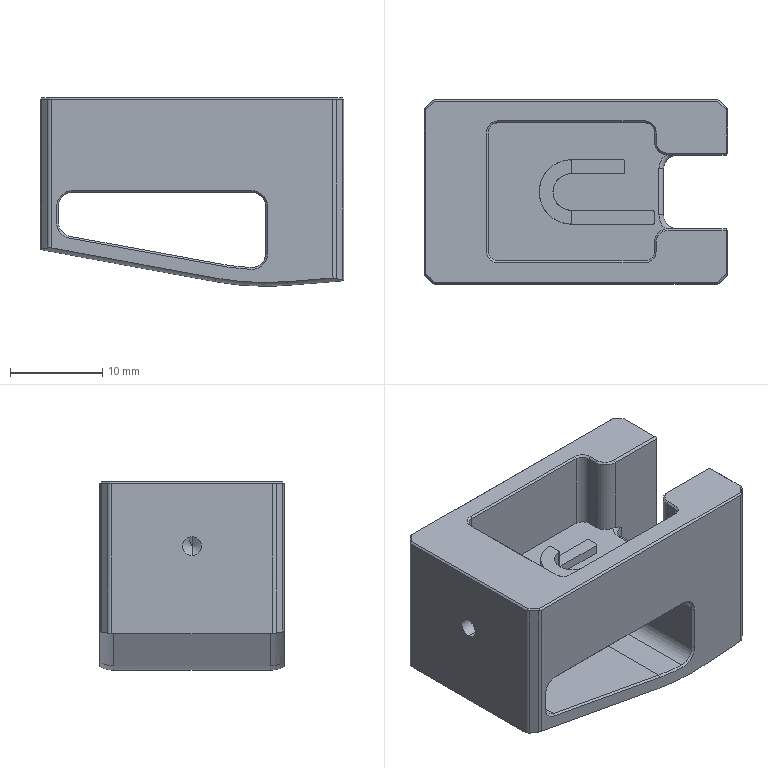NC program | NX | posted with a generic post | part box 33 x 20 x 20.478 mm
Lines 1 to 1297 of 7616:
N10 G17 G21 G94 G90
(CAVITY_MILL_1 , TOOL : D80)
N12 T19 M6
N14 G54
N16 G17 G0 G90 X95.922 Y-16.565 B0. C0. S6500 M3
N18 G43 Z30. H19
N20 Z7.
N22 G94 G1 Z4. F1500.
N24 X55.646
N26 X-55.646
N28 G2 X-56.192 Y-10.061 R39.693
N30 G1 X-56.196 Y-7.594
N32 Y7.594
N34 X-56.192 Y10.061
N36 G2 X-55.646 Y16.565 R39.693
N38 G1 X55.646
N40 X95.922
N42 Z7.
N44 G0 Z30.
N46 Y-16.565
N48 Z6.
N50 G1 Z3.
N52 X55.646
N54 X-55.646
N56 G2 X-56.192 Y-10.061 R39.693
N58 G1 X-56.196 Y-7.594
N60 Y7.594
N62 X-56.192 Y10.061
N64 G2 X-55.646 Y16.565 R39.693
N66 G1 X55.646
N68 X95.922
N70 Z6.
N72 G0 Z30.
N74 Y-16.565
N76 Z5.
N78 G1 Z2.
N80 X55.646
N82 X-55.646
N84 G2 X-56.193 Y-10.061 R39.693
N86 G1 X-56.196 Y-7.594
N88 Y7.594
N90 X-56.193 Y10.061
N92 G2 X-55.646 Y16.565 R39.693
N94 G1 X55.646
N96 X95.922
N98 Z5.
N100 G0 Z30.
N102 Y-16.565
N104 Z4.
N106 G1 Z1.
N108 X55.646
N110 X-55.646
N112 G2 X-56.193 Y-10.062 R39.693
N114 G1 X-56.196 Y-7.594
N116 Y7.594
N118 X-56.193 Y10.062
N120 G2 X-55.646 Y16.565 R39.693
N122 G1 X55.646
N124 X95.922
N126 Z4.
N128 G0 Z30.
N130 Y-16.565
N132 Z3.
N134 G1 Z0.
N136 X55.647
N138 X-55.647
N140 G2 X-56.193 Y-10.062 R39.693
N142 G1 X-56.197 Y-7.594
N144 Y7.594
N146 X-56.193 Y10.062
N148 G2 X-55.647 Y16.565 R39.693
N150 G1 X55.647
N152 X95.922
N154 Z3.
N156 G0 Z30.
N158 M5
(FIXED_CONTOUR , TOOL : D6)
N160 T12 M6
N162 G54
N164 G17 G0 G90 X-2.101 Y-13.027 B0. C0. S9500 M3
N166 G43 Z30. H12
N168 Z3.6
N170 G94 G1 Z2.384 F1000.
N172 X-2.171 Z1.918
N174 X-2.312 Z1.469
N176 X-2.522 Z1.048
N178 X-2.795 Z0.664
N180 X-3.125 Y-13.026 Z0.328
N182 X-3.503 Z0.048
N184 X-3.92 Z-0.17
N186 X-4.367 Y-13.025 Z-0.319
N188 X-4.831 Z-0.397
N190 X-5.302 Z-0.401
N192 X-5.692 Z-0.374 F2500.
N194 X-6.654 Y-13.024 Z-0.326
N196 X-7.492 Y-13.023 Z-0.305
N198 X-8.392 Z-0.304
N200 X-9.292 Y-13.022 Z-0.328
N202 X-9.487 Z-0.334
N204 X-11.092 Y-13.021 Z-0.439
N206 X-12.892 Y-13.019 Z-0.583
N208 X-14.692 Y-13.018 Z-0.728
N210 X-15.814 Y-13.017 Z-0.818
N212 X-15.995 Y-12.937 Z-0.787
N214 X-16.111 Y-12.868 Z-0.76
N216 X-16.222 Y-12.789 Z-0.733
N218 X-16.446 Y-12.623 Z-0.677
N220 X-16.548 Y-12.552 Z-0.654
N222 X-16.491 Z-0.65
N224 X-14.691 Y-12.553 Z-0.506
N226 X-12.891 Y-12.554 Z-0.362
N228 X-11.091 Y-12.556 Z-0.218
N230 X-10.191 Z-0.158
N232 X-9.291 Y-12.557 Z-0.115
N234 X-8.391 Z-0.091
N236 X-7.491 Y-12.558 Z-0.092
N238 X-6.591 Y-12.559 Z-0.116
N240 X-5.691 Z-0.158
N242 X-4.791 Y-12.56 Z-0.22
N244 X-3.891 Y-12.561 Z-0.309
N246 X-2.991 Z-0.421
N248 X-2.091 Y-12.562 Z-0.558
N250 X-0.291 Y-12.563 Z-0.878
N252 X1.509 Y-12.564 Z-1.21
N254 X3.309 Y-12.566 Z-1.541
N256 X5.109 Y-12.567 Z-1.872
N258 X6.909 Y-12.568 Z-2.203
N260 X8.709 Y-12.569 Z-2.533
N262 X10.509 Y-12.571 Z-2.864
N264 X12.309 Y-12.572 Z-3.195
N266 X14.109 Y-12.573 Z-3.525
N268 X15.909 Y-12.575 Z-3.856
N270 X16.876 Z-4.034
N272 X17.19 Y-12.346 Z-3.997
N274 X17.471 Y-12.138 Z-3.968
N276 X17.541 Y-12.083 Z-3.962
N278 X15.909 Y-12.082 Z-3.662
N280 X14.109 Y-12.081 Z-3.331
N282 X12.309 Y-12.08 Z-3.001
N284 X10.509 Y-12.078 Z-2.67
N286 X8.709 Y-12.077 Z-2.339
N288 X6.909 Y-12.076 Z-2.008
N290 X5.109 Y-12.074 Z-1.678
N292 X3.309 Y-12.073 Z-1.347
N294 X1.509 Y-12.072 Z-1.016
N296 X-0.291 Y-12.071 Z-0.685
N298 X-2.091 Y-12.069 Z-0.372
N300 X-2.991 Z-0.249
N302 X-3.891 Y-12.068 Z-0.149
N304 X-4.791 Z-0.07
N306 X-5.691 Y-12.067 Z-0.01
N308 X-7.491 Y-12.066 Z0.042
N310 X-8.391 Y-12.065 Z0.044
N312 X-9.291 Y-12.064 Z0.024
N314 X-10.191 Z-0.011
N316 X-11.091 Y-12.063 Z-0.068
N318 X-12.891 Y-12.062 Z-0.211
N320 X-14.691 Y-12.061 Z-0.355
N322 X-16.491 Y-12.059 Z-0.499
N324 X-17.269 Z-0.561
N326 X-17.674 Y-11.779 Z-0.535
N328 X-17.84 Y-11.652 Z-0.527
N330 X-17.942 Y-11.566 Z-0.522
N332 X-16.491 Y-11.567 Z-0.406
N334 X-14.691 Y-11.568 Z-0.261
N336 X-12.891 Y-11.569 Z-0.117
N338 X-11.091 Y-11.571 Z0.017
N340 X-9.291 Y-11.572 Z0.089
N342 X-7.491 Y-11.573 Z0.097
N344 X-6.591 Y-11.574 Z0.089
N346 X-5.691 Z0.06
N348 X-4.791 Y-11.575 Z0.018
N350 X-3.891 Y-11.576 Z-0.047
N352 X-2.991 Z-0.137
N354 X-2.091 Y-11.577 Z-0.251
N356 X-0.291 Y-11.578 Z-0.548
N358 X1.509 Y-11.579 Z-0.879
N360 X3.309 Y-11.581 Z-1.21
N362 X5.109 Y-11.582 Z-1.541
N364 X6.909 Y-11.583 Z-1.871
N366 X8.709 Y-11.585 Z-2.202
N368 X10.509 Y-11.586 Z-2.532
N370 X12.309 Y-11.587 Z-2.863
N372 X14.109 Y-11.588 Z-3.193
N374 X15.909 Y-11.59 Z-3.524
N376 X17.709 Y-11.591 Z-3.854
N378 X18.151 Z-3.936
N380 X18.373 Y-11.381 Z-3.929
N382 X18.575 Y-11.167 Z-3.924
N384 X18.631 Y-11.099 Z-3.922
N386 X17.71 Y-11.098 Z-3.753
N388 X15.91 Y-11.097 Z-3.423
N390 X14.11 Y-11.096 Z-3.092
N392 X12.31 Y-11.095 Z-2.762
N394 X10.51 Y-11.093 Z-2.431
N396 X8.71 Y-11.092 Z-2.101
N398 X6.91 Y-11.091 Z-1.77
N400 X5.11 Y-11.09 Z-1.44
N402 X3.31 Y-11.088 Z-1.109
N404 X1.51 Y-11.087 Z-0.779
N406 X-0.29 Y-11.086 Z-0.448
N408 X-1.19 Y-11.085 Z-0.297
N410 X-2.09 Y-11.084 Z-0.169
N412 X-2.99 Z-0.069
N414 X-3.89 Y-11.083 Z0.008
N416 X-4.79 Z0.062
N418 X-5.69 Y-11.082 Z0.091
N420 X-7.49 Y-11.081 Z0.099
N422 X-9.29 Y-11.079
N424 X-10.19 Z0.091
N426 X-11.09 Y-11.078 Z0.063
N428 X-12.89 Y-11.077 Z-0.06
N430 X-14.69 Y-11.076 Z-0.204
N432 X-16.49 Y-11.074 Z-0.348
N434 X-18.29 Y-11.073 Z-0.493
N436 X-18.439 Z-0.504
N438 X-18.508 Y-10.987 Z-0.502
N440 X-18.643 Y-10.801 Z-0.499
N442 X-18.724 Y-10.681 Z-0.496
N444 X-18.796 Y-10.58 Z-0.495
N446 X-18.29 Y-10.581 Z-0.454
N448 X-16.49 Y-10.582 Z-0.309
N450 X-14.69 Y-10.583 Z-0.165
N452 X-12.89 Y-10.584 Z-0.02
N454 X-11.99 Y-10.585 Z0.041
N456 X-11.09 Y-10.586 Z0.083
N458 X-10.19 Z0.098
N460 X-9.29 Y-10.587 Z0.099
N462 X-7.49 Y-10.588
N464 X-5.69 Y-10.59
N466 X-4.79 Z0.083
N468 X-3.89 Y-10.591 Z0.042
N470 X-2.99 Z-0.022
N472 X-2.09 Y-10.592 Z-0.113
N474 X-1.19 Y-10.593 Z-0.233
N476 X-0.29 Z-0.377
N478 X1.51 Y-10.595 Z-0.704
N480 X3.31 Y-10.596 Z-1.034
N482 X5.11 Y-10.597 Z-1.365
N484 X6.91 Y-10.598 Z-1.695
N486 X8.71 Y-10.6 Z-2.026
N488 X10.51 Y-10.601 Z-2.356
N490 X12.31 Y-10.602 Z-2.687
N492 X14.11 Y-10.603 Z-3.018
N494 X15.91 Y-10.605 Z-3.348
N496 X17.71 Y-10.606 Z-3.679
N498 X18.956 Y-10.607 Z-3.907
N500 X19.127 Y-10.287 Z-3.902
N502 X19.163 Y-10.196 Z-3.899
N504 X19.189 Y-10.115 Z-3.897
N506 X17.71 Y-10.113 Z-3.625
N508 X15.91 Y-10.112 Z-3.295
N510 X14.11 Y-10.111 Z-2.965
N512 X12.31 Y-10.11 Z-2.635
N514 X10.51 Y-10.108 Z-2.304
N516 X8.71 Y-10.107 Z-1.974
N518 X6.91 Y-10.106 Z-1.644
N520 X5.11 Y-10.105 Z-1.313
N522 X3.31 Y-10.103 Z-0.982
N524 X1.51 Y-10.102 Z-0.651
N526 X-0.29 Y-10.101 Z-0.328
N528 X-1.19 Y-10.1 Z-0.19
N530 X-2.09 Z-0.08
N532 X-2.99 Y-10.099 Z0.003
N534 X-3.89 Y-10.098 Z0.062
N536 X-4.79 Z0.092
N538 X-5.69 Y-10.097 Z0.099
N540 X-7.49 Y-10.096
N542 X-9.29 Y-10.095
N544 X-10.19 Y-10.094
N546 X-11.09 Y-10.093 Z0.093
N548 X-11.99 Z0.062
N550 X-12.89 Y-10.092 Z0.004
N552 X-14.69 Y-10.091 Z-0.138
N554 X-16.49 Y-10.089 Z-0.283
N556 X-18.29 Y-10.088 Z-0.427
N558 X-19.101 Z-0.492
N560 X-19.194 Y-9.729 Z-0.487
N562 X-19.234 Y-9.595 Z-0.486
N564 X-18.289 Y-9.596 Z-0.41
N566 X-16.489 Y-9.597 Z-0.265
N568 X-14.689 Y-9.598 Z-0.121
N570 X-12.889 Y-9.6 Z0.019
N572 X-11.989 Z0.073
N574 X-11.089 Y-9.601 Z0.097
N576 X-9.289 Y-9.602 Z0.099
N578 X-7.489 Y-9.603
N580 X-5.689 Y-9.605
N582 X-4.789 Z0.097
N584 X-3.889 Y-9.606 Z0.072
N586 X-2.989 Z0.019
N588 X-2.089 Y-9.607 Z-0.057
N590 X-1.189 Y-9.608 Z-0.162
N592 X-0.289 Z-0.294
N594 X1.511 Y-9.61 Z-0.614
N596 X3.311 Y-9.611 Z-0.944
N598 X5.111 Y-9.612 Z-1.275
N600 X6.911 Y-9.613 Z-1.605
N602 X8.711 Y-9.615 Z-1.936
N604 X10.511 Y-9.616 Z-2.266
N606 X12.311 Y-9.617 Z-2.597
N608 X14.111 Y-9.618 Z-2.927
N610 X15.911 Y-9.62 Z-3.258
N612 X17.711 Y-9.621 Z-3.588
N614 X19.336 Y-9.622 Z-3.886
N616 X19.428 Y-9.225 Z-3.884
N618 X19.439 Y-9.13 Z-3.883
N620 X17.711 Y-9.129 Z-3.566
N622 X15.911 Y-9.127 Z-3.235
N624 X14.111 Y-9.126 Z-2.905
N626 X12.311 Y-9.125 Z-2.575
N628 X10.511 Y-9.124 Z-2.244
N630 X8.711 Y-9.122 Z-1.914
N632 X6.911 Y-9.121 Z-1.584
N634 X5.111 Y-9.12 Z-1.254
N636 X3.311 Y-9.118 Z-0.923
N638 X1.511 Y-9.117 Z-0.593
N640 X-0.289 Y-9.116 Z-0.274
N642 X-1.189 Y-9.115 Z-0.144
N644 X-2.089 Z-0.042
N646 X-2.989 Y-9.114 Z0.029
N648 X-3.889 Y-9.113 Z0.078
N650 X-4.789 Z0.099
N652 X-5.689 Y-9.112
N654 X-7.489 Y-9.111
N656 X-9.289 Y-9.11
N658 X-11.089 Y-9.108 Z0.098
N660 X-11.989 Z0.079
N662 X-12.889 Y-9.107 Z0.029
N664 X-14.689 Y-9.106 Z-0.109
N666 X-16.489 Y-9.105 Z-0.254
N668 X-18.289 Y-9.103 Z-0.399
N670 X-19.371 Z-0.486
N672 X-19.482 Y-8.61 Z-0.49
N674 X-18.289 Y-8.611 Z-0.394
N676 X-16.489 Y-8.612 Z-0.249
N678 X-14.689 Y-8.613 Z-0.105
N680 X-12.889 Y-8.615 Z0.033
N682 X-11.989 Z0.081
N684 X-11.089 Y-8.616 Z0.098
N686 X-9.289 Y-8.617 Z0.099
N688 X-7.489 Y-8.618
N690 X-5.689 Y-8.62
N692 X-4.789
N694 X-3.889 Y-8.621 Z0.08
N696 X-2.989 Y-8.622 Z0.033
N698 X-2.089 Z-0.036
N700 X-1.189 Y-8.623 Z-0.137
N702 X-0.289 Z-0.264
N704 X1.511 Y-8.625 Z-0.582
N706 X3.311 Y-8.626 Z-0.912
N708 X5.111 Y-8.627 Z-1.242
N710 X6.911 Y-8.629 Z-1.573
N712 X8.711 Y-8.63 Z-1.903
N714 X10.511 Y-8.631 Z-2.234
N716 X12.311 Y-8.632 Z-2.564
N718 X14.111 Y-8.634 Z-2.895
N720 X15.911 Y-8.635 Z-3.225
N722 X17.711 Y-8.636 Z-3.555
N724 X19.491 Y-8.637 Z-3.882
N726 X19.512 Y-8.254 Z-3.885
N728 Y-8.145
N730 X0.499 Y-8.132 Z-0.395
N732 X-0.288 Y-8.131 Z-0.264
N734 X-1.188 Y-8.13 Z-0.136
N736 X-2.088 Z-0.035
N738 X-2.988 Y-8.129 Z0.033
N740 X-3.888 Y-8.128 Z0.08
N742 X-4.788 Z0.099
N744 X-5.688 Y-8.127
N746 X-7.488 Y-8.126
N748 X-9.288 Y-8.125
N750 X-11.088 Y-8.123 Z0.098
N752 X-11.988 Z0.081
N754 X-12.888 Y-8.122 Z0.033
N756 X-13.359 Z0.003
N758 X-19.508 Y-8.117 Z-0.492
N760 Y-7.625
N762 X-13.359 Y-7.629 Z0.003
N764 X-12.888 Y-7.63 Z0.033
N766 X-11.988 Z0.081
N768 X-11.088 Y-7.631 Z0.098
N770 X-9.288 Y-7.632 Z0.099
N772 X-7.488 Y-7.633
N774 X-5.688 Y-7.635
N776 X-4.788
N778 X-3.888 Y-7.636 Z0.08
N780 X-2.988 Y-7.637 Z0.033
N782 X-2.088 Z-0.036
N784 X-1.188 Y-7.638 Z-0.136
N786 X-0.288 Y-7.639 Z-0.264
N788 X0.5 Z-0.395
N790 X19.512 Y-7.652 Z-3.885
N792 Y-7.16
N794 X0.5 Y-7.147 Z-0.396
N796 X-0.288 Y-7.146 Z-0.264
N798 X-1.188 Y-7.145 Z-0.136
N800 X-2.088 Z-0.036
N802 X-2.988 Y-7.144 Z0.033
N804 X-3.888 Z0.08
N806 X-4.788 Y-7.143 Z0.099
N808 X-5.688 Y-7.142
N810 X-7.488 Y-7.141
N812 X-9.288 Y-7.14
N814 X-11.088 Y-7.138 Z0.098
N816 X-11.988 Z0.081
N818 X-12.888 Y-7.137 Z0.033
N820 X-13.359 Z0.003
N822 X-19.507 Y-7.133 Z-0.492
N824 Y-6.64
N826 X-13.358 Y-6.644 Z0.003
N828 X-12.887 Y-6.645 Z0.033
N830 X-11.987 Z0.081
N832 X-11.087 Y-6.646 Z0.098
N834 X-9.287 Y-6.647 Z0.099
N836 X-7.487 Y-6.649
N838 X-5.687 Y-6.65
N840 X-4.787
N842 X-3.887 Y-6.651 Z0.08
N844 X-2.987 Y-6.652 Z0.033
N846 X-2.087 Z-0.036
N848 X-1.187 Y-6.653 Z-0.136
N850 X-0.287 Y-6.654 Z-0.264
N852 X0.5 Z-0.396
N854 X19.512 Y-6.668 Z-3.885
N856 Y-6.175
N858 X0.501 Y-6.162 Z-0.396
N860 X-0.287 Y-6.161 Z-0.264
N862 X-1.187 Z-0.137
N864 X-2.087 Y-6.16 Z-0.036
N866 X-2.987 Y-6.159 Z0.033
N868 X-3.887 Z0.08
N870 X-4.787 Y-6.158 Z0.099
N872 X-5.687 Y-6.157
N874 X-7.487 Y-6.156
N876 X-9.287 Y-6.155
N878 X-11.087 Y-6.154 Z0.098
N880 X-11.987 Y-6.153 Z0.081
N882 X-12.887 Y-6.152 Z0.033
N884 X-13.358 Z0.003
N886 X-19.507 Y-6.148 Z-0.492
N888 Y-5.655
N890 X-13.358 Y-5.66 Z0.003
N892 X-12.887 Z0.032
N894 X-11.987 Z0.081
N896 X-11.087 Y-5.661 Z0.098
N898 X-9.287 Y-5.662 Z0.099
N900 X-7.487 Y-5.664
N902 X-5.687 Y-5.665
N904 X-4.787 Y-5.666
N906 X-3.887 Z0.08
N908 X-2.987 Y-5.667 Z0.033
N910 X-2.087 Z-0.036
N912 X-1.187 Y-5.668 Z-0.137
N914 X-0.287 Y-5.669 Z-0.264
N916 X0.501 Z-0.396
N918 X19.512 Y-5.683 Z-3.885
N920 Y-5.19
N922 X0.501 Y-5.177 Z-0.396
N924 X-0.286 Y-5.176 Z-0.264
N926 X-1.186 Z-0.137
N928 X-2.086 Y-5.175 Z-0.036
N930 X-2.986 Y-5.174 Z0.033
N932 X-3.886 Z0.08
N934 X-4.786 Y-5.173 Z0.099
N936 X-5.686 Y-5.172
N938 X-7.486 Y-5.171
N940 X-9.286 Y-5.17
N942 X-11.086 Y-5.169 Z0.098
N944 X-11.986 Y-5.168 Z0.081
N946 X-12.886 Y-5.167 Z0.034
N948 X-13.357 Z0.003
N950 X-19.507 Y-5.163 Z-0.492
N952 X-19.506 Y-4.855
N954 X-19.502 Y-4.67
N956 X-13.357 Y-4.675 Z0.003
N958 X-12.886 Z0.036
N960 X-11.986 Y-4.676 Z0.082
N962 X-11.086 Z0.098
N964 X-9.286 Y-4.677 Z0.099
N966 X-7.486 Y-4.679
N968 X-5.686 Y-4.68
N970 X-4.786 Y-4.681
N972 X-3.886 Z0.08
N974 X-2.986 Y-4.682 Z0.033
N976 X-2.086 Y-4.683 Z-0.036
N978 X-1.186 Z-0.137
N980 X-0.286 Y-4.684 Z-0.264
N982 X0.502 Z-0.396
N984 X19.512 Y-4.698 Z-3.885
N986 Y-4.205
N988 X0.502 Y-4.192 Z-0.396
N990 X-0.286 Y-4.191 Z-0.264
N992 X-1.186 Z-0.137
N994 X-2.086 Y-4.19 Z-0.036
N996 X-2.986 Y-4.189 Z0.033
N998 X-3.886 Z0.08
N1000 X-4.786 Y-4.188 Z0.099
N1002 X-5.686
N1004 X-7.486 Y-4.186
N1006 X-9.286 Y-4.185
N1008 X-11.086 Y-4.184 Z0.098
N1010 X-11.986 Y-4.183 Z0.082
N1012 X-12.886 Y-4.182 Z0.037
N1014 X-13.448 Z-0.006
N1016 X-14.686 Y-4.181 Z-0.106
N1018 X-16.486 Y-4.18 Z-0.251
N1020 X-18.286 Y-4.179 Z-0.395
N1022 X-19.478 Y-4.178 Z-0.491
N1024 X-19.473 Y-4.126 Z-0.492
N1026 X-19.43 Y-3.884
N1028 X-19.376 Y-3.685 Z-0.491
N1030 X-18.285 Y-3.686 Z-0.404
N1032 X-16.485 Y-3.687 Z-0.259
N1034 X-14.685 Y-3.689 Z-0.114
N1036 X-13.785 Z-0.041
N1038 X-12.885 Y-3.69 Z0.034
N1040 X-11.985 Y-3.691 Z0.082
N1042 X-11.085 Z0.098
N1044 X-9.285 Y-3.693 Z0.099
N1046 X-7.485 Y-3.694
N1048 X-5.685 Y-3.695
N1050 X-4.785 Y-3.696
N1052 X-3.885 Z0.08
N1054 X-2.985 Y-3.697 Z0.033
N1056 X-2.085 Y-3.698 Z-0.036
N1058 X-1.185 Z-0.137
N1060 X-0.285 Y-3.699 Z-0.265
N1062 X0.495 Z-0.395
N1064 X19.512 Y-3.713 Z-3.885
N1066 Y-3.22
N1068 X0.496 Y-3.207 Z-0.395
N1070 X-0.285 Y-3.206 Z-0.265
N1072 X-1.185 Z-0.137
N1074 X-2.085 Y-3.205 Z-0.036
N1076 X-2.985 Y-3.204 Z0.033
N1078 X-3.885 Z0.08
N1080 X-4.785 Y-3.203 Z0.099
N1082 X-5.685
N1084 X-7.485 Y-3.201
N1086 X-9.285 Y-3.2
N1088 X-11.085 Y-3.199 Z0.098
N1090 X-11.985 Y-3.198 Z0.082
N1092 X-12.885 Z0.023
N1094 X-12.99 Y-3.197 Z0.013
N1096 X-13.095 Z0.003
N1098 X-13.757 Z-0.055
N1100 X-14.685 Y-3.196 Z-0.13
N1102 X-16.485 Y-3.195 Z-0.274
N1104 X-18.285 Y-3.194 Z-0.419
N1106 X-19.178 Y-3.193 Z-0.491
N1108 X-19.127 Y-3.084 Z-0.492
N1110 X-19.023 Y-2.913 Z-0.491
N1112 X-18.867 Y-2.701
N1114 X-18.285 Z-0.444
N1116 X-16.485 Y-2.703 Z-0.299
N1118 X-14.685 Y-2.704 Z-0.154
N1120 X-13.335 Y-2.705 Z-0.046
N1122 X-12.885 Z-0.004
N1124 X-12.819 Z0.003
N1126 X-12.627 Z0.024
N1128 X-12.435 Z0.044
N1130 X-11.985 Y-2.706 Z0.082
N1132 X-11.085 Z0.098
N1134 X-9.285 Y-2.708 Z0.099
N1136 X-7.485 Y-2.709
N1138 X-5.685 Y-2.71
N1140 X-4.785 Y-2.711
N1142 X-3.885 Z0.08
N1144 X-2.985 Y-2.712 Z0.032
N1146 X-2.085 Y-2.713 Z-0.036
N1148 X-1.185 Z-0.137
N1150 X-0.285 Y-2.714 Z-0.265
N1152 X0.496 Z-0.395
N1154 X19.512 Y-2.728 Z-3.885
N1156 Y-2.235
N1158 X0.496 Y-2.222 Z-0.395
N1160 X-0.284 Y-2.221 Z-0.265
N1162 X-1.184 Z-0.137
N1164 X-2.084 Y-2.22 Z-0.036
N1166 X-2.984 Z0.032
N1168 X-3.884 Y-2.219 Z0.08
N1170 X-4.784 Y-2.218 Z0.099
N1172 X-5.684
N1174 X-7.484 Y-2.216
N1176 X-9.284 Y-2.215
N1178 X-11.084 Y-2.214 Z0.098
N1180 X-11.744 Y-2.213 Z0.088
N1182 X-11.992 Z0.081
N1184 X-12.045 Z0.056
N1186 X-12.074 Z0.051
N1188 X-12.239 Z0.025
N1190 X-12.404 Z0.002
N1192 X-12.884 Z-0.048
N1194 X-14.684 Y-2.211 Z-0.193
N1196 X-16.484 Y-2.21 Z-0.338
N1198 X-18.284 Y-2.209 Z-0.483
N1200 X-18.375 Z-0.49
N1202 X-18.159 Y-2.031 Z-0.492
N1204 X-18.024 Y-1.942
N1206 X-17.674 Y-1.77
N1208 X-17.53 Y-1.717 Z-0.49
N1210 X-16.484 Y-1.718 Z-0.406
N1212 X-14.684 Y-1.719 Z-0.261
N1214 X-12.884 Y-1.72 Z-0.116
N1216 X-12.158 Y-1.721 Z-0.058
N1218 X-12.091 Z0.01
N1220 X-12.049 Z0.052
N1222 X-12.041 Z0.059
N1224 X-12.024 Z0.07
N1226 X-11.99 Z0.081
N1228 X-11.621 Z0.091
N1230 X-11.084 Z0.098
N1232 X-9.284 Y-1.723 Z0.099
N1234 X-7.484 Y-1.724
N1236 X-5.684 Y-1.725
N1238 X-4.784 Y-1.726
N1240 X-3.884 Z0.08
N1242 X-2.984 Y-1.727 Z0.032
N1244 X-2.084 Y-1.728 Z-0.036
N1246 X-1.184 Z-0.137
N1248 X-0.284 Y-1.729 Z-0.265
N1250 X0.497 Y-1.73 Z-0.395
N1252 X19.512 Y-1.743 Z-3.885
N1254 Y-1.25
N1256 X0.497 Y-1.237 Z-0.395
N1258 X-0.283 Z-0.265
N1260 X-1.183 Y-1.236 Z-0.137
N1262 X-2.083 Y-1.235 Z-0.036
N1264 X-2.983 Z0.032
N1266 X-3.883 Y-1.234 Z0.08
N1268 X-4.783 Y-1.233 Z0.099
N1270 X-5.683
N1272 X-7.483 Y-1.231
N1274 X-9.283 Y-1.23
N1276 X-11.083 Y-1.229 Z0.098
N1278 X-11.805 Y-1.228 Z0.086
N1280 X-11.986 Z0.082
N1282 X-12.031 Z0.067
N1284 X-12.053 Z0.048
N1286 X-12.527 Z-0.426
N1288 X-16.733 Y-1.225 Z-0.767
N1290 X-16.682 Y-1.005 Z-0.977
N1292 X-16.494 Y-0.951 Z-1.014
N1294 X-12.6 Y-0.941 Z-0.711
N1296 X-12.597 Y-1.149 Z-0.508
N1298 X-12.571 Y-1.189 Z-0.468
N1300 Y-1.186 Z-0.47
N1302 Y-0.735
N1304 X-12.052 Y-0.736 Z0.049
N1306 X-12.046 Z0.054
N1308 X-12. Z0.079
N1310 X-11.977 Z0.082
N1312 X-11.955 Z0.083
N1314 X-11.083 Y-0.737 Z0.098
N1316 X-9.283 Y-0.738 Z0.099
N1318 X-7.483 Y-0.739
N1320 X-5.683 Y-0.74
N1322 X-4.783 Y-0.741
N1324 X-3.883 Y-0.742 Z0.08
N1326 X-2.983 Z0.032
N1328 X-2.083 Y-0.743 Z-0.036
N1330 X-1.183 Z-0.137
N1332 X-0.283 Y-0.744 Z-0.265
N1334 X0.497 Y-0.745 Z-0.395
N1336 X19.512 Y-0.758 Z-3.885
N1338 Y-0.266
N1340 X0.498 Y-0.252 Z-0.395
N1342 X-0.283 Z-0.265
N1344 X-1.183 Y-0.251 Z-0.137
N1346 X-2.083 Y-0.25 Z-0.036
N1348 X-2.983 Z0.032
N1350 X-3.883 Y-0.249 Z0.08
N1352 X-4.783 Y-0.248 Z0.099
N1354 X-5.683
N1356 X-7.483 Y-0.247
N1358 X-9.283 Y-0.245
N1360 X-11.083 Y-0.244 Z0.098
N1362 X-11.977 Y-0.243 Z0.082
N1364 X-12. Z0.079
N1366 X-12.046 Z0.055
N1368 X-12.052 Z0.049
N1370 X-12.566 Z-0.465
N1372 X-12.571 Z-0.47
N1374 Y0.249
N1376 X-12.052 Z0.049
N1378 X-12.046 Z0.055
N1380 X-12. Z0.079
N1382 X-11.977 Z0.082
N1384 X-11.954 Z0.083
N1386 X-11.082 Y0.248 Z0.098
N1388 X-9.282 Y0.247 Z0.099
N1390 X-7.482 Y0.246
N1392 X-5.682 Y0.245
N1394 X-4.782 Y0.244
N1396 X-3.882 Y0.243 Z0.08
N1398 X-2.982 Z0.032
N1400 X-2.082 Y0.242 Z-0.036
N1402 X-1.182 Y0.241 Z-0.137
N1404 X-0.282 Z-0.265
N1406 X0.498 Y0.24 Z-0.395
N1408 X19.512 Y0.227 Z-3.885
N1410 Y0.719
N1412 X0.498 Y0.733 Z-0.395
N1414 X-0.282 Z-0.265
N1416 X-1.182 Y0.734 Z-0.137
N1418 X-2.082 Y0.735 Z-0.036
N1420 X-2.982 Z0.032
N1422 X-3.882 Y0.736 Z0.08
N1424 X-4.782 Z0.099
N1426 X-5.682 Y0.737
N1428 X-7.482 Y0.738
N1430 X-9.282 Y0.74
N1432 X-11.082 Y0.741 Z0.098
N1434 X-11.977 Y0.742 Z0.082
N1436 X-12. Z0.079
N1438 X-12.046 Z0.055
N1440 X-12.052 Z0.049
N1442 X-12.566 Z-0.465
N1444 X-12.571 Z-0.47
N1446 Y1.147
N1448 X-12.574 Y1.183 Z-0.473
N1450 X-12.577 Y1.196 Z-0.462
N1452 X-12.597 Y1.139 Z-0.518
N1454 X-12.6 Y0.941 Z-0.711
N1456 X-16.403 Y0.948 Z-1.009
N1458 X-16.677 Y0.988 Z-0.994
N1460 X-16.735 Y1.237 Z-0.755
N1462 X-12.52 Y1.234 Z-0.419
N1464 X-12.048 Z0.053
N1466 X-12.026 Z0.07
N1468 X-12.003 Z0.079
N1470 X-11.992 Z0.081
N1472 X-11.981 Z0.082
N1474 X-11.801 Z0.086
N1476 X-11.082 Y1.233 Z0.098
N1478 X-9.282 Y1.232 Z0.099
N1480 X-7.482 Y1.231
N1482 X-5.682 Y1.23
N1484 X-4.782 Y1.229
N1486 X-3.882 Y1.228 Z0.08
N1488 X-2.982 Z0.032
N1490 X-2.082 Y1.227 Z-0.036
N1492 X-1.182 Y1.226 Z-0.137
N1494 X-0.282 Z-0.265
N1496 X0.499 Y1.225 Z-0.395
N1498 X19.512 Y1.212 Z-3.885
N1500 Y1.704
N1502 X0.499 Y1.718 Z-0.395
N1504 X-0.281 Z-0.265
N1506 X-1.181 Y1.719 Z-0.137
N1508 X-2.081 Z-0.036
N1510 X-2.981 Y1.72 Z0.032
N1512 X-3.881 Y1.721 Z0.08
N1514 X-4.781 Z0.099
N1516 X-5.681 Y1.722
N1518 X-7.481 Y1.723
N1520 X-9.281 Y1.725
N1522 X-11.081 Y1.726 Z0.098
N1524 X-11.981 Z0.082
N1526 X-12.025 Z0.07
N1528 X-12.047 Z0.054
N1530 X-12.053 Z0.048
N1532 X-12.157 Y1.727 Z-0.056
N1534 X-12.881 Z-0.114
N1536 X-14.681 Y1.728 Z-0.259
N1538 X-16.481 Y1.73 Z-0.403
N1540 X-17.572 Z-0.491
N1542 X-17.674 Y1.767 Z-0.492
N1544 X-17.851 Y1.849
N1546 X-18.025 Y1.942
N1548 X-18.159 Y2.028
N1550 X-18.41 Y2.223 Z-0.491
N1552 X-18.281 Z-0.481
N1554 X-16.481 Y2.222 Z-0.336
N1556 X-14.681 Y2.221 Z-0.192
N1558 X-12.881 Y2.22 Z-0.047
N1560 X-12.431 Y2.219 Z-0.001
N1562 X-12.392 Z0.005
N1564 X-12.206 Z0.03
N1566 X-12.094 Z0.048
N1568 X-12.044 Z0.057
N1570 X-12.037 Z0.062
N1572 X-11.981 Z0.082
N1574 X-11.081 Y2.218 Z0.098
N1576 X-9.281 Y2.217 Z0.099
N1578 X-7.481 Y2.216
N1580 X-5.681 Y2.214
N1582 X-4.781
N1584 X-3.881 Y2.213 Z0.08
N1586 X-2.981 Z0.032
N1588 X-2.081 Y2.212 Z-0.036
N1590 X-1.181 Y2.211 Z-0.137
N1592 X-0.281 Z-0.265
N1594 X0.499 Y2.21 Z-0.395
N1596 X19.512 Y2.197 Z-3.885
N1598 Y2.689
N1600 X0.5 Y2.703 Z-0.395
N1602 X-0.281 Z-0.265
N1604 X-1.181 Y2.704 Z-0.137
N1606 X-2.081 Z-0.036
N1608 X-2.981 Y2.705 Z0.032
N1610 X-3.881 Y2.706 Z0.08
N1612 X-4.781 Z0.099
N1614 X-5.681 Y2.707
N1616 X-7.481 Y2.708
N1618 X-9.281 Y2.709
N1620 X-11.081 Y2.711 Z0.098
N1622 X-12.009 Z0.081
N1624 X-12.206 Y2.712 Z0.066
N1626 X-12.81 Z0.005
N1628 X-12.881 Z-0.003
N1630 X-14.681 Y2.713 Z-0.153
N1632 X-16.481 Y2.715 Z-0.298
N1634 X-18.281 Y2.716 Z-0.443
N1636 X-18.879 Z-0.491
N1638 X-19.023 Y2.913
N1640 X-19.127 Y3.083 Z-0.492
N1642 X-19.191 Y3.209
N1644 X-18.28 Y3.208 Z-0.418
N1646 X-16.48 Y3.207 Z-0.274
N1648 X-14.68 Y3.206 Z-0.129
N1650 X-13.78 Y3.205 Z-0.056
N1652 X-13.33 Z-0.018
N1654 X-12.88 Y3.204 Z0.023
N1656 X-12.43 Z0.06
N1658 X-12.093 Z0.078
N1660 X-11.98 Z0.082
N1662 X-11.08 Y3.203 Z0.098
N1664 X-9.28 Y3.202 Z0.099
N1666 X-7.48 Y3.201
N1668 X-5.68 Y3.199
N1670 X-4.78
N1672 X-3.88 Y3.198 Z0.08
N1674 X-2.98 Y3.197 Z0.032
N1676 X-2.08 Z-0.036
N1678 X-1.18 Y3.196 Z-0.137
N1680 X-0.28 Z-0.265
N1682 X0.5 Y3.195 Z-0.396
N1684 X19.512 Y3.182 Z-3.885
N1686 Y3.674
N1688 X0.5 Y3.688 Z-0.396
N1690 X-0.28 Z-0.265
N1692 X-1.18 Y3.689 Z-0.137
N1694 X-2.08 Z-0.036
N1696 X-2.98 Y3.69 Z0.032
N1698 X-3.88 Y3.691 Z0.08
N1700 X-4.78 Z0.099
N1702 X-5.68 Y3.692
N1704 X-7.48 Y3.693
N1706 X-9.28 Y3.694
N1708 X-11.08 Y3.696 Z0.098
N1710 X-11.98 Z0.081
N1712 X-12.43 Y3.697 Z0.063
N1714 X-12.88 Z0.034
N1716 X-13.78 Y3.698 Z-0.041
N1718 X-14.68 Z-0.113
N1720 X-16.48 Y3.699 Z-0.258
N1722 X-18.28 Y3.701 Z-0.403
N1724 X-19.38 Z-0.491
N1726 X-19.43 Y3.884 Z-0.492
N1728 X-19.473 Y4.126
N1730 X-19.479 Y4.194 Z-0.491
N1732 X-18.28 Y4.193 Z-0.395
N1734 X-16.48 Y4.192 Z-0.25
N1736 X-14.68 Y4.191 Z-0.105
N1738 X-13.105 Y4.19 Z0.022
N1740 X-12.88 Y4.189 Z0.037
N1742 X-11.98 Z0.081
N1744 X-11.08 Y4.188 Z0.098
N1746 X-9.28 Y4.187 Z0.099
N1748 X-7.48 Y4.186
N1750 X-5.68 Y4.184
N1752 X-4.78
N1754 X-3.88 Y4.183 Z0.08
N1756 X-2.98 Y4.182 Z0.032
N1758 X-2.08 Z-0.036
N1760 X-1.18 Y4.181 Z-0.137
N1762 X-0.28 Z-0.265
N1764 X0.501 Y4.18 Z-0.396
N1766 X19.512 Y4.167 Z-3.885
N1768 Y4.659
N1770 X0.501 Y4.672 Z-0.396
N1772 X-0.279 Y4.673 Z-0.266
N1774 X-1.179 Y4.674 Z-0.138
N1776 X-2.079 Z-0.036
N1778 X-2.979 Y4.675 Z0.032
N1780 X-3.879 Z0.08
N1782 X-4.779 Y4.676 Z0.099
N1784 X-5.679 Y4.677
N1786 X-7.479 Y4.678
N1788 X-9.279 Y4.679
N1790 X-11.079 Y4.681 Z0.098
N1792 X-11.979 Z0.081
N1794 X-12.879 Y4.682 Z0.036
N1796 X-13.357 Z0.003
N1798 X-19.502 Y4.686 Z-0.492
N1800 X-19.506 Y4.855
N1802 X-19.507 Y5.179
N1804 X-13.357 Y5.175 Z0.003
N1806 X-12.879 Y5.174 Z0.035
N1808 X-11.979 Z0.081
N1810 X-11.079 Y5.173 Z0.098
N1812 X-9.279 Y5.172 Z0.099
N1814 X-7.479 Y5.17
N1816 X-5.679 Y5.169
N1818 X-4.779
N1820 X-3.879 Y5.168 Z0.08
N1822 X-2.979 Y5.167 Z0.032
N1824 X-2.079 Z-0.036
N1826 X-1.179 Y5.166 Z-0.138
N1828 X-0.279 Y5.165 Z-0.266
N1830 X0.501 Z-0.396
N1832 X19.512 Y5.152 Z-3.885
N1834 Y5.644
N1836 X0.502 Y5.657 Z-0.396
N1838 X-0.279 Y5.658 Z-0.266
N1840 X-1.179 Y5.659 Z-0.138
N1842 X-2.079 Z-0.037
N1844 X-2.979 Y5.66 Z0.032
N1846 X-3.879 Z0.08
N1848 X-4.779 Y5.661 Z0.099
N1850 X-5.679 Y5.662
N1852 X-7.479 Y5.663
N1854 X-9.279 Y5.664
N1856 X-11.079 Y5.665 Z0.098
N1858 X-11.979 Y5.666 Z0.081
N1860 X-12.879 Y5.667 Z0.034
N1862 X-13.357 Z0.003
N1864 X-19.507 Y5.671 Z-0.492
N1866 Y6.164
N1868 X-13.356 Y6.16 Z0.003
N1870 X-12.878 Y6.159 Z0.034
N1872 X-11.978 Z0.081
N1874 X-11.078 Y6.158 Z0.098
N1876 X-9.278 Y6.157 Z0.099
N1878 X-7.478 Y6.155
N1880 X-5.678 Y6.154
N1882 X-4.778
N1884 X-3.878 Y6.153 Z0.08
N1886 X-2.978 Y6.152 Z0.032
N1888 X-2.078 Z-0.037
N1890 X-1.178 Y6.151 Z-0.138
N1892 X-0.278 Y6.15 Z-0.266
N1894 X0.495 Z-0.395
N1896 X19.512 Y6.136 Z-3.885
N1898 Y6.629
N1900 X0.495 Y6.642 Z-0.395
N1902 X-0.278 Y6.643 Z-0.266
N1904 X-1.178 Z-0.138
N1906 X-2.078 Y6.644 Z-0.037
N1908 X-2.978 Y6.645 Z0.032
N1910 X-3.878 Z0.08
N1912 X-4.778 Y6.646 Z0.099
N1914 X-5.678 Y6.647
N1916 X-7.478 Y6.648
N1918 X-9.278 Y6.649
N1920 X-11.078 Y6.65 Z0.098
N1922 X-11.978 Y6.651 Z0.081
N1924 X-12.878 Y6.652 Z0.033
N1926 X-13.356 Z0.003
N1928 X-19.507 Y6.656 Z-0.492
N1930 Y7.149
N1932 X-13.356 Y7.144 Z0.003
N1934 X-12.878 Z0.034
N1936 X-11.978 Y7.143 Z0.081
N1938 X-11.078 Z0.098
N1940 X-9.278 Y7.142 Z0.099
N1942 X-7.478 Y7.14
N1944 X-5.678 Y7.139
N1946 X-4.778 Y7.138
N1948 X-3.878 Z0.08
N1950 X-2.978 Y7.137 Z0.032
N1952 X-2.078 Z-0.037
N1954 X-1.178 Y7.136 Z-0.138
N1956 X-0.278 Y7.135 Z-0.266
N1958 X0.496 Z-0.395
N1960 X19.512 Y7.121 Z-3.885
N1962 Y7.614
N1964 X0.496 Y7.627 Z-0.395
N1966 X-0.277 Y7.628 Z-0.266
N1968 X-1.177 Z-0.138
N1970 X-2.077 Y7.629 Z-0.037
N1972 X-2.977 Y7.63 Z0.032
N1974 X-3.877 Z0.08
N1976 X-4.777 Y7.631 Z0.099
N1978 X-5.677 Y7.632
N1980 X-7.477 Y7.633
N1982 X-9.277 Y7.634
N1984 X-11.077 Y7.635 Z0.098
N1986 X-11.977 Y7.636 Z0.081
N1988 X-12.877 Y7.637 Z0.034
N1990 X-13.355 Z0.003
N1992 X-19.508 Y7.641 Z-0.492
N1994 Y8.134
N1996 X-13.355 Y8.129 Z0.003
N1998 X-12.877 Z0.034
N2000 X-11.977 Y8.128 Z0.081
N2002 X-11.077 Z0.098
N2004 X-9.277 Y8.127 Z0.099
N2006 X-7.477 Y8.125
N2008 X-5.677 Y8.124
N2010 X-4.777 Y8.123
N2012 X-3.877 Z0.08
N2014 X-2.977 Y8.122 Z0.032
N2016 X-2.077 Y8.121 Z-0.037
N2018 X-1.177 Z-0.138
N2020 X-0.277 Y8.12 Z-0.266
N2022 X0.497 Z-0.395
N2024 X19.512 Y8.106 Z-3.885
N2026 Y8.254
N2028 X19.493 Y8.599 Z-3.882
N2030 X17.723 Y8.6 Z-3.557
N2032 X15.923 Y8.601 Z-3.227
N2034 X14.123 Y8.603 Z-2.897
N2036 X12.323 Y8.604 Z-2.566
N2038 X10.523 Y8.605 Z-2.236
N2040 X8.723 Y8.606 Z-1.905
N2042 X6.923 Y8.608 Z-1.575
N2044 X5.123 Y8.609 Z-1.245
N2046 X3.323 Y8.61 Z-0.914
N2048 X1.523 Y8.611 Z-0.584
N2050 X-0.277 Y8.613 Z-0.266
N2052 X-1.177 Z-0.138
N2054 X-2.077 Y8.614 Z-0.037
N2056 X-2.977 Y8.615 Z0.032
N2058 X-3.877 Z0.08
N2060 X-4.777 Y8.616 Z0.099
N2062 X-5.677
N2064 X-7.477 Y8.618
N2066 X-9.277 Y8.619
N2068 X-11.077 Y8.62 Z0.098
N2070 X-11.977 Y8.621 Z0.081
N2072 X-12.877 Y8.622 Z0.033
N2074 X-14.677 Y8.623 Z-0.104
N2076 X-16.477 Y8.624 Z-0.248
N2078 X-18.277 Y8.625 Z-0.393
N2080 X-19.478 Y8.626 Z-0.49
N2082 X-19.367 Y9.119 Z-0.486
N2084 X-18.276 Y9.118 Z-0.398
N2086 X-16.476 Y9.116 Z-0.253
N2088 X-14.676 Y9.115 Z-0.108
N2090 X-12.876 Y9.114 Z0.03
N2092 X-11.976 Y9.113 Z0.08
N2094 X-11.076 Z0.098
N2096 X-9.276 Y9.111 Z0.099
N2098 X-7.476 Y9.11
N2100 X-5.676 Y9.109
N2102 X-4.776 Y9.108
N2104 X-3.876 Z0.077
N2106 X-2.976 Y9.107 Z0.028
N2108 X-2.076 Y9.106 Z-0.043
N2110 X-1.176 Z-0.146
N2112 X-0.276 Y9.105 Z-0.276
N2114 X1.524 Y9.104 Z-0.595
N2116 X3.324 Y9.103 Z-0.925
N2118 X5.124 Y9.101 Z-1.255
N2120 X6.924 Y9.1 Z-1.586
N2122 X8.724 Y9.099 Z-1.916
N2124 X10.524 Y9.098 Z-2.246
N2126 X12.324 Y9.096 Z-2.576
N2128 X14.124 Y9.095 Z-2.907
N2130 X15.924 Y9.094 Z-3.237
N2132 X17.724 Y9.092 Z-3.567
N2134 X19.444 Y9.091 Z-3.883
N2136 X19.428 Y9.225 Z-3.884
N2138 X19.345 Y9.584 Z-3.886
N2140 X17.724 Y9.585 Z-3.588
N2142 X15.924 Y9.586 Z-3.258
N2144 X14.124 Y9.587 Z-2.928
N2146 X12.324 Y9.589 Z-2.597
N2148 X10.524 Y9.59 Z-2.267
N2150 X8.724 Y9.591 Z-1.937
N2152 X6.924 Y9.593 Z-1.606
N2154 X5.124 Y9.594 Z-1.276
N2156 X3.324 Y9.595 Z-0.946
N2158 X1.524 Y9.596 Z-0.615
N2160 X-0.276 Y9.598 Z-0.296
N2162 X-1.176 Z-0.164
N2164 X-2.076 Y9.599 Z-0.058
N2166 X-2.976 Z0.018
N2168 X-3.876 Y9.6 Z0.071
N2170 X-4.776 Y9.601 Z0.096
N2172 X-5.676 Z0.099
N2174 X-7.476 Y9.603
N2176 X-9.276 Y9.604
N2178 X-11.076 Y9.605 Z0.097
N2180 X-11.976 Y9.606 Z0.074
N2182 X-12.876 Z0.02
N2184 X-14.676 Y9.608 Z-0.12
N2186 X-16.476 Y9.609 Z-0.265
N2188 X-18.276 Y9.61 Z-0.409
N2190 X-19.228 Y9.611 Z-0.486
N2192 X-19.199 Y9.71
N2194 X-19.097 Y10.103 Z-0.493
N2196 X-18.276 Z-0.427
N2198 X-16.476 Y10.101 Z-0.282
N2200 X-14.676 Y10.1 Z-0.138
N2202 X-12.876 Y10.099 Z0.005
N2204 X-11.976 Y10.098 Z0.062
N2206 X-11.076 Z0.093
N2208 X-10.176 Y10.097 Z0.099
N2210 X-9.276 Y10.096
N2212 X-7.476 Y10.095
N2214 X-5.676 Y10.094
N2216 X-4.776 Y10.093 Z0.092
N2218 X-3.876 Z0.062
N2220 X-2.976 Y10.092 Z0.002
N2222 X-2.076 Y10.091 Z-0.081
N2224 X-1.176 Z-0.192
N2226 X-0.276 Y10.09 Z-0.33
N2228 X1.524 Y10.089 Z-0.653
N2230 X3.324 Y10.088 Z-0.983
N2232 X5.124 Y10.086 Z-1.314
N2234 X6.924 Y10.085 Z-1.644
N2236 X8.724 Y10.084 Z-1.975
N2238 X10.524 Y10.082 Z-2.305
N2240 X12.324 Y10.081 Z-2.635
N2242 X14.124 Y10.08 Z-2.965
N2244 X15.924 Y10.079 Z-3.295
N2246 X17.724 Y10.077 Z-3.625
N2248 X19.201 Y10.076 Z-3.895
N2250 X19.163 Y10.196 Z-3.899
N2252 X19.127 Y10.287 Z-3.902
N2254 X18.976 Y10.569 Z-3.907
N2256 X17.725 Y10.57 Z-3.677
N2258 X15.925 Y10.571 Z-3.347
N2260 X14.125 Y10.572 Z-3.016
N2262 X12.325 Y10.574 Z-2.686
N2264 X10.525 Y10.575 Z-2.356
N2266 X8.725 Y10.576 Z-2.026
N2268 X6.925 Y10.577 Z-1.695
N2270 X5.125 Y10.579 Z-1.365
N2272 X3.325 Y10.58 Z-1.035
N2274 X1.525 Y10.581 Z-0.705
N2276 X-0.275 Y10.582 Z-0.379
N2278 X-1.175 Y10.583 Z-0.234
N2280 X-2.075 Y10.584 Z-0.114
N2282 X-2.975 Z-0.023
N2284 X-3.875 Y10.585 Z0.041
N2286 X-4.775 Y10.586 Z0.082
N2288 X-5.675 Z0.099
N2290 X-7.475 Y10.588
N2292 X-9.275 Y10.589
N2294 X-10.175 Z0.098
N2296 X-11.075 Y10.59 Z0.083
N2298 X-11.975 Y10.591 Z0.042
N2300 X-12.875 Z-0.019
N2302 X-14.675 Y10.593 Z-0.164
N2304 X-16.475 Y10.594 Z-0.309
N2306 X-18.275 Y10.595 Z-0.454
N2308 X-18.793 Y10.596 Z-0.496
N2310 X-18.508 Y10.987 Z-0.502
N2312 X-18.427 Y11.088 Z-0.505
N2314 X-18.275 Z-0.493
N2316 X-16.475 Y11.086 Z-0.348
N2318 X-14.675 Y11.085 Z-0.204
N2320 X-12.875 Y11.084 Z-0.059
N2322 X-11.075 Y11.083 Z0.064
N2324 X-10.175 Y11.082 Z0.091
N2326 X-9.275 Y11.081 Z0.099
N2328 X-7.475 Y11.08
N2330 X-5.675 Y11.079 Z0.091
N2332 X-4.775 Y11.078 Z0.062
N2334 X-3.875 Y11.077 Z0.007
N2336 X-2.975 Z-0.07
N2338 X-2.075 Y11.076 Z-0.17
N2340 X-1.175 Z-0.298
N2342 X-0.275 Y11.075 Z-0.449
N2344 X1.525 Y11.074 Z-0.779
N2346 X3.325 Y11.072 Z-1.109
N2348 X5.125 Y11.071 Z-1.439
N2350 X6.925 Y11.07 Z-1.77
N2352 X8.725 Y11.069 Z-2.1
N2354 X10.525 Y11.067 Z-2.43
N2356 X12.325 Y11.066 Z-2.76
N2358 X14.125 Y11.065 Z-3.09
N2360 X15.925 Y11.064 Z-3.42
N2362 X17.725 Y11.062 Z-3.75
N2364 X18.659 Z-3.921
N2366 X18.643 Y11.085 Z-3.922
N2368 X18.575 Y11.167 Z-3.924
N2370 X18.373 Y11.381 Z-3.929
N2372 X18.19 Y11.554 Z-3.934
N2374 X17.726 Y11.555 Z-3.849
N2376 X15.926 Y11.556 Z-3.519
N2378 X14.126 Y11.557 Z-3.189
N2380 X12.326 Y11.559 Z-2.859
N2382 X10.526 Y11.56 Z-2.529
N2384 X8.726 Y11.561 Z-2.199
N2386 X6.926 Y11.562 Z-1.869
N2388 X5.126 Y11.564 Z-1.539
N2390 X3.326 Y11.565 Z-1.209
N2392 X1.526 Y11.566 Z-0.879
N2394 X-0.274 Y11.567 Z-0.549
N2396 X-2.074 Y11.569 Z-0.252
N2398 X-2.974 Z-0.138
N2400 X-3.874 Y11.57 Z-0.048
N2402 X-4.774 Y11.571 Z0.017
N2404 X-5.674 Z0.06
N2406 X-6.574 Y11.572 Z0.089
N2408 X-7.474 Z0.097
N2410 X-9.274 Y11.574 Z0.09
N2412 X-11.074 Y11.575 Z0.018
N2414 X-12.874 Y11.576 Z-0.116
N2416 X-14.674 Y11.578 Z-0.261
N2418 X-16.474 Y11.579 Z-0.406
N2420 X-17.925 Y11.58 Z-0.523
N2422 X-17.84 Y11.652 Z-0.527
N2424 X-17.674 Y11.779 Z-0.535
N2426 X-17.25 Y12.072 Z-0.563
N2428 X-16.474 Y12.071 Z-0.5
N2430 X-14.674 Y12.07 Z-0.356
N2432 X-12.874 Y12.069 Z-0.211
N2434 X-11.074 Y12.067 Z-0.068
N2436 X-10.174 Z-0.01
N2438 X-9.274 Y12.066 Z0.024
N2440 X-8.374 Z0.044
N2442 X-7.474 Y12.065 Z0.042
N2444 X-5.674 Y12.064 Z-0.01
N2446 X-4.774 Y12.063 Z-0.07
N2448 X-3.874 Y12.062 Z-0.149
N2450 X-2.974 Z-0.249
N2452 X-2.074 Y12.061 Z-0.372
N2454 X-0.274 Y12.06 Z-0.685
N2456 X1.526 Y12.059 Z-1.016
N2458 X3.326 Y12.057 Z-1.347
N2460 X5.126 Y12.056 Z-1.678
N2462 X6.926 Y12.055 Z-2.008
N2464 X8.726 Y12.054 Z-2.338
N2466 X10.526 Y12.052 Z-2.668
N2468 X12.326 Y12.051 Z-2.998
N2470 X14.126 Y12.05 Z-3.328
N2472 X15.926 Y12.048 Z-3.658
N2474 X17.584 Y12.047 Z-3.962
N2476 X17.19 Y12.347 Z-3.994
N2478 X16.924 Y12.54 Z-4.03
N2480 X15.926 Y12.541 Z-3.847
N2482 X14.126 Y12.542 Z-3.517
N2484 X12.326 Y12.543 Z-3.187
N2486 X10.526 Y12.545 Z-2.857
N2488 X8.726 Y12.546 Z-2.527
N2490 X6.926 Y12.547 Z-2.197
N2492 X5.126 Y12.549 Z-1.867
N2494 X3.326 Y12.55 Z-1.537
N2496 X1.526 Y12.551 Z-1.207
N2498 X-0.274 Y12.552 Z-0.877
N2500 X-2.074 Y12.554 Z-0.557
N2502 X-2.974 Z-0.42
N2504 X-3.874 Y12.555 Z-0.309
N2506 X-4.774 Z-0.22
N2508 X-5.674 Y12.556 Z-0.158
N2510 X-6.574 Y12.557 Z-0.116
N2512 X-7.474 Z-0.092
N2514 X-8.374 Y12.558 Z-0.091
N2516 X-9.274 Y12.559 Z-0.115
N2518 X-10.174 Z-0.158
N2520 X-11.074 Y12.56 Z-0.218
N2522 X-12.874 Y12.561 Z-0.363
N2524 X-14.674 Y12.562 Z-0.508
N2526 X-16.474 Y12.564 Z-0.653
N2528 X-16.531 Z-0.657
N2530 X-16.446 Y12.623 Z-0.677
N2532 X-16.222 Y12.787 Z-0.732
N2534 X-15.998 Y12.941 Z-0.79
N2536 X-15.938 Y12.981 Z-0.807
N2538 X-15.737 Y13.009
N2540 X-15.253 Y13.021 Z-0.774
N2542 X-14.673 Y13.02 Z-0.727
N2544 X-12.873 Y13.019 Z-0.582
N2546 X-11.073 Y13.018 Z-0.436
N2548 X-9.8 Y13.017 Z-0.349
N2550 X-9.273 Z-0.324
N2552 X-8.373 Y13.016 Z-0.3
N2554 X-7.473 Y13.015 Z-0.301
N2556 X-5.858 Y13.014 Z-0.359
N2558 X-5.673 Z-0.37
N2560 X-4.777 Y13.013 Z-0.44
N2562 X-4.306 Z-0.439
N2564 X-3.841 Z-0.365
N2566 X-3.394 Z-0.22
N2568 X-2.975 Y13.012 Z-0.006
N2570 X-2.594 Z0.271
N2572 X-2.261 Z0.605
N2574 X-1.985 Z0.986
N2576 X-1.772 Y13.011 Z1.405
N2578 X-1.626 Z1.853
N2580 X-1.553 Z2.318
N2582 Z3.6
N2584 G0 Z30.
N2586 M5